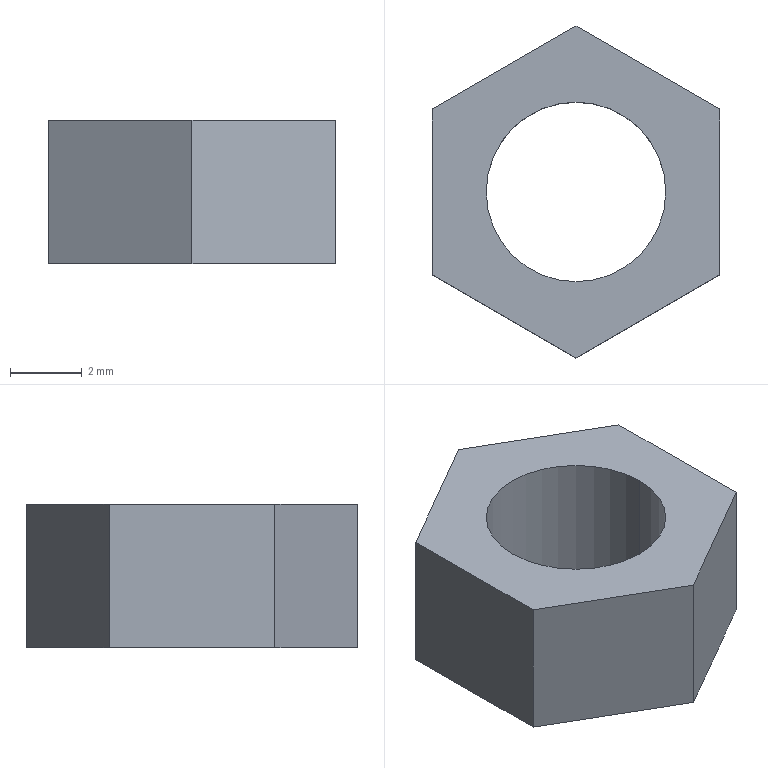Part | STEP file | M5 nut | 1 solid | 10 faces | box 8 x 9.238 x 4 mm | volume 143.163 mm3 | plane 8 | cylinder 2 | commonest cylinder face diameters 5 x2
STEP:
#1=CARTESIAN_POINT('',(0.,0.,0.));
#2=DIRECTION('',(0.,0.,1.));
#3=DIRECTION('',(1.,0.,0.));
#4=AXIS2_PLACEMENT_3D('',#1,#2,#3);
#5=CARTESIAN_POINT('',(2.5,0.,0.));
#6=VERTEX_POINT('',#5);
#7=CARTESIAN_POINT('',(2.5,0.,4.));
#8=VERTEX_POINT('',#7);
#9=CARTESIAN_POINT('',(2.5,0.,0.));
#10=DIRECTION('',(0.,0.,1.));
#11=VECTOR('',#10,1.);
#12=LINE('',#9,#11);
#13=CARTESIAN_POINT('',(0.,0.,0.));
#14=DIRECTION('',(0.,0.,1.));
#15=DIRECTION('',(1.,0.,0.));
#16=AXIS2_PLACEMENT_3D('',#13,#14,#15);
#17=CYLINDRICAL_SURFACE('',#16,2.5);
#18=CARTESIAN_POINT('',(6.283,0.));
#19=DIRECTION('',(0.,1.));
#20=VECTOR('',#19,1.);
#21=LINE('',#18,#20);
#22=(GEOMETRIC_REPRESENTATION_CONTEXT(2)PARAMETRIC_REPRESENTATION_CONTEXT()REPRESENTATION_CONTEXT('',''));
#23=DEFINITIONAL_REPRESENTATION('',(#21),#22);
#24=PCURVE('',#17,#23);
#25=CARTESIAN_POINT('',(0.,0.,0.));
#26=DIRECTION('',(0.,0.,1.));
#27=DIRECTION('',(1.,0.,0.));
#28=AXIS2_PLACEMENT_3D('',#25,#26,#27);
#29=CYLINDRICAL_SURFACE('',#28,2.5);
#30=CARTESIAN_POINT('',(0.,0.));
#31=DIRECTION('',(0.,1.));
#32=VECTOR('',#31,1.);
#33=LINE('',#30,#32);
#34=(GEOMETRIC_REPRESENTATION_CONTEXT(2)PARAMETRIC_REPRESENTATION_CONTEXT()REPRESENTATION_CONTEXT('',''));
#35=DEFINITIONAL_REPRESENTATION('',(#33),#34);
#36=PCURVE('',#29,#35);
#37=SURFACE_CURVE('',#12,(#24,#36),.PCURVE_S1.);
#38=EDGE_CURVE('',#6,#8,#37,.T.);
#39=ORIENTED_EDGE('',*,*,#38,.T.);
#40=CARTESIAN_POINT('',(-2.5,0.,4.));
#41=VERTEX_POINT('',#40);
#42=CARTESIAN_POINT('',(0.,0.,4.));
#43=DIRECTION('',(0.,0.,1.));
#44=DIRECTION('',(1.,0.,0.));
#45=AXIS2_PLACEMENT_3D('',#42,#43,#44);
#46=CIRCLE('',#45,2.5);
#47=CARTESIAN_POINT('',(0.,4.));
#48=DIRECTION('',(1.,0.));
#49=VECTOR('',#48,1.);
#50=LINE('',#47,#49);
#51=(GEOMETRIC_REPRESENTATION_CONTEXT(2)PARAMETRIC_REPRESENTATION_CONTEXT()REPRESENTATION_CONTEXT('',''));
#52=DEFINITIONAL_REPRESENTATION('',(#50),#51);
#53=PCURVE('',#17,#52);
#54=CARTESIAN_POINT('',(0.,0.,4.));
#55=DIRECTION('',(0.,0.,1.));
#56=DIRECTION('',(1.,0.,0.));
#57=AXIS2_PLACEMENT_3D('',#54,#55,#56);
#58=PLANE('',#57);
#59=CARTESIAN_POINT('',(0.,0.));
#60=DIRECTION('',(1.,0.));
#61=AXIS2_PLACEMENT_2D('',#59,#60);
#62=CIRCLE('',#61,2.5);
#63=(GEOMETRIC_REPRESENTATION_CONTEXT(2)PARAMETRIC_REPRESENTATION_CONTEXT()REPRESENTATION_CONTEXT('',''));
#64=DEFINITIONAL_REPRESENTATION('',(#62),#63);
#65=PCURVE('',#58,#64);
#66=SURFACE_CURVE('',#46,(#53,#65),.PCURVE_S1.);
#67=EDGE_CURVE('',#41,#8,#66,.T.);
#68=ORIENTED_EDGE('',*,*,#67,.F.);
#69=CARTESIAN_POINT('',(-2.5,0.,0.));
#70=VERTEX_POINT('',#69);
#71=CARTESIAN_POINT('',(-2.5,0.,0.));
#72=DIRECTION('',(0.,0.,1.));
#73=VECTOR('',#72,1.);
#74=LINE('',#71,#73);
#75=CARTESIAN_POINT('',(3.142,0.));
#76=DIRECTION('',(0.,1.));
#77=VECTOR('',#76,1.);
#78=LINE('',#75,#77);
#79=(GEOMETRIC_REPRESENTATION_CONTEXT(2)PARAMETRIC_REPRESENTATION_CONTEXT()REPRESENTATION_CONTEXT('',''));
#80=DEFINITIONAL_REPRESENTATION('',(#78),#79);
#81=PCURVE('',#17,#80);
#82=CARTESIAN_POINT('',(3.142,0.));
#83=DIRECTION('',(0.,1.));
#84=VECTOR('',#83,1.);
#85=LINE('',#82,#84);
#86=(GEOMETRIC_REPRESENTATION_CONTEXT(2)PARAMETRIC_REPRESENTATION_CONTEXT()REPRESENTATION_CONTEXT('',''));
#87=DEFINITIONAL_REPRESENTATION('',(#85),#86);
#88=PCURVE('',#29,#87);
#89=SURFACE_CURVE('',#74,(#81,#88),.PCURVE_S1.);
#90=EDGE_CURVE('',#70,#41,#89,.T.);
#91=ORIENTED_EDGE('',*,*,#90,.F.);
#92=CARTESIAN_POINT('',(0.,0.,0.));
#93=DIRECTION('',(0.,0.,1.));
#94=DIRECTION('',(1.,0.,0.));
#95=AXIS2_PLACEMENT_3D('',#92,#93,#94);
#96=CIRCLE('',#95,2.5);
#97=CARTESIAN_POINT('',(0.,0.));
#98=DIRECTION('',(1.,0.));
#99=VECTOR('',#98,1.);
#100=LINE('',#97,#99);
#101=(GEOMETRIC_REPRESENTATION_CONTEXT(2)PARAMETRIC_REPRESENTATION_CONTEXT()REPRESENTATION_CONTEXT('',''));
#102=DEFINITIONAL_REPRESENTATION('',(#100),#101);
#103=PCURVE('',#17,#102);
#104=CARTESIAN_POINT('',(0.,0.,0.));
#105=DIRECTION('',(0.,0.,1.));
#106=DIRECTION('',(1.,0.,0.));
#107=AXIS2_PLACEMENT_3D('',#104,#105,#106);
#108=PLANE('',#107);
#109=CARTESIAN_POINT('',(0.,0.));
#110=DIRECTION('',(1.,0.));
#111=AXIS2_PLACEMENT_2D('',#109,#110);
#112=CIRCLE('',#111,2.5);
#113=(GEOMETRIC_REPRESENTATION_CONTEXT(2)PARAMETRIC_REPRESENTATION_CONTEXT()REPRESENTATION_CONTEXT('',''));
#114=DEFINITIONAL_REPRESENTATION('',(#112),#113);
#115=PCURVE('',#108,#114);
#116=SURFACE_CURVE('',#96,(#103,#115),.PCURVE_S1.);
#117=EDGE_CURVE('',#70,#6,#116,.T.);
#118=ORIENTED_EDGE('',*,*,#117,.T.);
#119=EDGE_LOOP('',(#39,#68,#91,#118));
#120=FACE_BOUND('',#119,.F.);
#121=ADVANCED_FACE('',(#120),#17,.F.);
#122=CARTESIAN_POINT('',(-4.,2.309,0.));
#123=VERTEX_POINT('',#122);
#124=CARTESIAN_POINT('',(-4.,-2.309,0.));
#125=VERTEX_POINT('',#124);
#126=CARTESIAN_POINT('',(-4.,2.309,0.));
#127=DIRECTION('',(0.,-1.,0.));
#128=VECTOR('',#127,1.);
#129=LINE('',#126,#128);
#130=CARTESIAN_POINT('',(-4.,2.309,4.));
#131=DIRECTION('',(1.,0.,0.));
#132=DIRECTION('',(0.,0.,-1.));
#133=AXIS2_PLACEMENT_3D('',#130,#131,#132);
#134=PLANE('',#133);
#135=CARTESIAN_POINT('',(4.,0.));
#136=DIRECTION('',(0.,-1.));
#137=VECTOR('',#136,1.);
#138=LINE('',#135,#137);
#139=(GEOMETRIC_REPRESENTATION_CONTEXT(2)PARAMETRIC_REPRESENTATION_CONTEXT()REPRESENTATION_CONTEXT('',''));
#140=DEFINITIONAL_REPRESENTATION('',(#138),#139);
#141=PCURVE('',#134,#140);
#142=CARTESIAN_POINT('',(-4.,2.309));
#143=DIRECTION('',(0.,-1.));
#144=VECTOR('',#143,1.);
#145=LINE('',#142,#144);
#146=(GEOMETRIC_REPRESENTATION_CONTEXT(2)PARAMETRIC_REPRESENTATION_CONTEXT()REPRESENTATION_CONTEXT('',''));
#147=DEFINITIONAL_REPRESENTATION('',(#145),#146);
#148=PCURVE('',#108,#147);
#149=SURFACE_CURVE('',#129,(#141,#148),.PCURVE_S1.);
#150=EDGE_CURVE('',#123,#125,#149,.T.);
#151=ORIENTED_EDGE('',*,*,#150,.T.);
#152=CARTESIAN_POINT('',(-4.,-2.309,4.));
#153=VERTEX_POINT('',#152);
#154=CARTESIAN_POINT('',(-4.,-2.309,4.));
#155=DIRECTION('',(0.,0.,-1.));
#156=VECTOR('',#155,1.);
#157=LINE('',#154,#156);
#158=CARTESIAN_POINT('',(0.,-4.619));
#159=DIRECTION('',(1.,0.));
#160=VECTOR('',#159,1.);
#161=LINE('',#158,#160);
#162=(GEOMETRIC_REPRESENTATION_CONTEXT(2)PARAMETRIC_REPRESENTATION_CONTEXT()REPRESENTATION_CONTEXT('',''));
#163=DEFINITIONAL_REPRESENTATION('',(#161),#162);
#164=PCURVE('',#134,#163);
#165=CARTESIAN_POINT('',(-4.,-2.309,4.));
#166=DIRECTION('',(0.5,0.866,0.));
#167=DIRECTION('',(-0.866,0.5,0.));
#168=AXIS2_PLACEMENT_3D('',#165,#166,#167);
#169=PLANE('',#168);
#170=CARTESIAN_POINT('',(0.,0.));
#171=DIRECTION('',(0.,-1.));
#172=VECTOR('',#171,1.);
#173=LINE('',#170,#172);
#174=(GEOMETRIC_REPRESENTATION_CONTEXT(2)PARAMETRIC_REPRESENTATION_CONTEXT()REPRESENTATION_CONTEXT('',''));
#175=DEFINITIONAL_REPRESENTATION('',(#173),#174);
#176=PCURVE('',#169,#175);
#177=SURFACE_CURVE('',#157,(#164,#176),.PCURVE_S1.);
#178=EDGE_CURVE('',#153,#125,#177,.T.);
#179=ORIENTED_EDGE('',*,*,#178,.F.);
#180=CARTESIAN_POINT('',(-4.,2.309,4.));
#181=VERTEX_POINT('',#180);
#182=CARTESIAN_POINT('',(-4.,2.309,4.));
#183=DIRECTION('',(0.,-1.,0.));
#184=VECTOR('',#183,1.);
#185=LINE('',#182,#184);
#186=CARTESIAN_POINT('',(0.,0.));
#187=DIRECTION('',(0.,-1.));
#188=VECTOR('',#187,1.);
#189=LINE('',#186,#188);
#190=(GEOMETRIC_REPRESENTATION_CONTEXT(2)PARAMETRIC_REPRESENTATION_CONTEXT()REPRESENTATION_CONTEXT('',''));
#191=DEFINITIONAL_REPRESENTATION('',(#189),#190);
#192=PCURVE('',#134,#191);
#193=CARTESIAN_POINT('',(-4.,2.309));
#194=DIRECTION('',(0.,-1.));
#195=VECTOR('',#194,1.);
#196=LINE('',#193,#195);
#197=(GEOMETRIC_REPRESENTATION_CONTEXT(2)PARAMETRIC_REPRESENTATION_CONTEXT()REPRESENTATION_CONTEXT('',''));
#198=DEFINITIONAL_REPRESENTATION('',(#196),#197);
#199=PCURVE('',#58,#198);
#200=SURFACE_CURVE('',#185,(#192,#199),.PCURVE_S1.);
#201=EDGE_CURVE('',#181,#153,#200,.T.);
#202=ORIENTED_EDGE('',*,*,#201,.F.);
#203=CARTESIAN_POINT('',(-4.,2.309,4.));
#204=DIRECTION('',(0.,0.,-1.));
#205=VECTOR('',#204,1.);
#206=LINE('',#203,#205);
#207=CARTESIAN_POINT('',(0.,0.));
#208=DIRECTION('',(1.,0.));
#209=VECTOR('',#208,1.);
#210=LINE('',#207,#209);
#211=(GEOMETRIC_REPRESENTATION_CONTEXT(2)PARAMETRIC_REPRESENTATION_CONTEXT()REPRESENTATION_CONTEXT('',''));
#212=DEFINITIONAL_REPRESENTATION('',(#210),#211);
#213=PCURVE('',#134,#212);
#214=CARTESIAN_POINT('',(0.,4.619,4.));
#215=DIRECTION('',(0.5,-0.866,0.));
#216=DIRECTION('',(0.866,0.5,0.));
#217=AXIS2_PLACEMENT_3D('',#214,#215,#216);
#218=PLANE('',#217);
#219=CARTESIAN_POINT('',(-4.619,0.));
#220=DIRECTION('',(0.,-1.));
#221=VECTOR('',#220,1.);
#222=LINE('',#219,#221);
#223=(GEOMETRIC_REPRESENTATION_CONTEXT(2)PARAMETRIC_REPRESENTATION_CONTEXT()REPRESENTATION_CONTEXT('',''));
#224=DEFINITIONAL_REPRESENTATION('',(#222),#223);
#225=PCURVE('',#218,#224);
#226=SURFACE_CURVE('',#206,(#213,#225),.PCURVE_S1.);
#227=EDGE_CURVE('',#181,#123,#226,.T.);
#228=ORIENTED_EDGE('',*,*,#227,.T.);
#229=EDGE_LOOP('',(#151,#179,#202,#228));
#230=FACE_BOUND('',#229,.T.);
#231=ADVANCED_FACE('',(#230),#134,.F.);
#232=CARTESIAN_POINT('',(0.,-4.619,0.));
#233=VERTEX_POINT('',#232);
#234=CARTESIAN_POINT('',(-4.,-2.309,0.));
#235=DIRECTION('',(0.866,-0.5,0.));
#236=VECTOR('',#235,1.);
#237=LINE('',#234,#236);
#238=CARTESIAN_POINT('',(0.,-4.));
#239=DIRECTION('',(-1.,0.));
#240=VECTOR('',#239,1.);
#241=LINE('',#238,#240);
#242=(GEOMETRIC_REPRESENTATION_CONTEXT(2)PARAMETRIC_REPRESENTATION_CONTEXT()REPRESENTATION_CONTEXT('',''));
#243=DEFINITIONAL_REPRESENTATION('',(#241),#242);
#244=PCURVE('',#169,#243);
#245=CARTESIAN_POINT('',(-4.,-2.309));
#246=DIRECTION('',(0.866,-0.5));
#247=VECTOR('',#246,1.);
#248=LINE('',#245,#247);
#249=(GEOMETRIC_REPRESENTATION_CONTEXT(2)PARAMETRIC_REPRESENTATION_CONTEXT()REPRESENTATION_CONTEXT('',''));
#250=DEFINITIONAL_REPRESENTATION('',(#248),#249);
#251=PCURVE('',#108,#250);
#252=SURFACE_CURVE('',#237,(#244,#251),.PCURVE_S1.);
#253=EDGE_CURVE('',#125,#233,#252,.T.);
#254=ORIENTED_EDGE('',*,*,#253,.T.);
#255=CARTESIAN_POINT('',(0.,-4.619,4.));
#256=VERTEX_POINT('',#255);
#257=CARTESIAN_POINT('',(0.,-4.619,4.));
#258=DIRECTION('',(0.,0.,-1.));
#259=VECTOR('',#258,1.);
#260=LINE('',#257,#259);
#261=CARTESIAN_POINT('',(-4.619,0.));
#262=DIRECTION('',(0.,-1.));
#263=VECTOR('',#262,1.);
#264=LINE('',#261,#263);
#265=(GEOMETRIC_REPRESENTATION_CONTEXT(2)PARAMETRIC_REPRESENTATION_CONTEXT()REPRESENTATION_CONTEXT('',''));
#266=DEFINITIONAL_REPRESENTATION('',(#264),#265);
#267=PCURVE('',#169,#266);
#268=CARTESIAN_POINT('',(0.,-4.619,4.));
#269=DIRECTION('',(-0.5,0.866,0.));
#270=DIRECTION('',(-0.866,-0.5,0.));
#271=AXIS2_PLACEMENT_3D('',#268,#269,#270);
#272=PLANE('',#271);
#273=CARTESIAN_POINT('',(0.,0.));
#274=DIRECTION('',(0.,-1.));
#275=VECTOR('',#274,1.);
#276=LINE('',#273,#275);
#277=(GEOMETRIC_REPRESENTATION_CONTEXT(2)PARAMETRIC_REPRESENTATION_CONTEXT()REPRESENTATION_CONTEXT('',''));
#278=DEFINITIONAL_REPRESENTATION('',(#276),#277);
#279=PCURVE('',#272,#278);
#280=SURFACE_CURVE('',#260,(#267,#279),.PCURVE_S1.);
#281=EDGE_CURVE('',#256,#233,#280,.T.);
#282=ORIENTED_EDGE('',*,*,#281,.F.);
#283=CARTESIAN_POINT('',(-4.,-2.309,4.));
#284=DIRECTION('',(0.866,-0.5,0.));
#285=VECTOR('',#284,1.);
#286=LINE('',#283,#285);
#287=CARTESIAN_POINT('',(0.,0.));
#288=DIRECTION('',(-1.,0.));
#289=VECTOR('',#288,1.);
#290=LINE('',#287,#289);
#291=(GEOMETRIC_REPRESENTATION_CONTEXT(2)PARAMETRIC_REPRESENTATION_CONTEXT()REPRESENTATION_CONTEXT('',''));
#292=DEFINITIONAL_REPRESENTATION('',(#290),#291);
#293=PCURVE('',#169,#292);
#294=CARTESIAN_POINT('',(-4.,-2.309));
#295=DIRECTION('',(0.866,-0.5));
#296=VECTOR('',#295,1.);
#297=LINE('',#294,#296);
#298=(GEOMETRIC_REPRESENTATION_CONTEXT(2)PARAMETRIC_REPRESENTATION_CONTEXT()REPRESENTATION_CONTEXT('',''));
#299=DEFINITIONAL_REPRESENTATION('',(#297),#298);
#300=PCURVE('',#58,#299);
#301=SURFACE_CURVE('',#286,(#293,#300),.PCURVE_S1.);
#302=EDGE_CURVE('',#153,#256,#301,.T.);
#303=ORIENTED_EDGE('',*,*,#302,.F.);
#304=ORIENTED_EDGE('',*,*,#178,.T.);
#305=EDGE_LOOP('',(#254,#282,#303,#304));
#306=FACE_BOUND('',#305,.T.);
#307=ADVANCED_FACE('',(#306),#169,.F.);
#308=CARTESIAN_POINT('',(4.,-2.309,0.));
#309=VERTEX_POINT('',#308);
#310=CARTESIAN_POINT('',(0.,-4.619,0.));
#311=DIRECTION('',(0.866,0.5,0.));
#312=VECTOR('',#311,1.);
#313=LINE('',#310,#312);
#314=CARTESIAN_POINT('',(0.,-4.));
#315=DIRECTION('',(-1.,0.));
#316=VECTOR('',#315,1.);
#317=LINE('',#314,#316);
#318=(GEOMETRIC_REPRESENTATION_CONTEXT(2)PARAMETRIC_REPRESENTATION_CONTEXT()REPRESENTATION_CONTEXT('',''));
#319=DEFINITIONAL_REPRESENTATION('',(#317),#318);
#320=PCURVE('',#272,#319);
#321=CARTESIAN_POINT('',(0.,-4.619));
#322=DIRECTION('',(0.866,0.5));
#323=VECTOR('',#322,1.);
#324=LINE('',#321,#323);
#325=(GEOMETRIC_REPRESENTATION_CONTEXT(2)PARAMETRIC_REPRESENTATION_CONTEXT()REPRESENTATION_CONTEXT('',''));
#326=DEFINITIONAL_REPRESENTATION('',(#324),#325);
#327=PCURVE('',#108,#326);
#328=SURFACE_CURVE('',#313,(#320,#327),.PCURVE_S1.);
#329=EDGE_CURVE('',#233,#309,#328,.T.);
#330=ORIENTED_EDGE('',*,*,#329,.T.);
#331=CARTESIAN_POINT('',(4.,-2.309,4.));
#332=VERTEX_POINT('',#331);
#333=CARTESIAN_POINT('',(4.,-2.309,4.));
#334=DIRECTION('',(0.,0.,-1.));
#335=VECTOR('',#334,1.);
#336=LINE('',#333,#335);
#337=CARTESIAN_POINT('',(-4.619,0.));
#338=DIRECTION('',(0.,-1.));
#339=VECTOR('',#338,1.);
#340=LINE('',#337,#339);
#341=(GEOMETRIC_REPRESENTATION_CONTEXT(2)PARAMETRIC_REPRESENTATION_CONTEXT()REPRESENTATION_CONTEXT('',''));
#342=DEFINITIONAL_REPRESENTATION('',(#340),#341);
#343=PCURVE('',#272,#342);
#344=CARTESIAN_POINT('',(4.,-2.309,4.));
#345=DIRECTION('',(-1.,0.,0.));
#346=DIRECTION('',(0.,0.,1.));
#347=AXIS2_PLACEMENT_3D('',#344,#345,#346);
#348=PLANE('',#347);
#349=CARTESIAN_POINT('',(0.,0.));
#350=DIRECTION('',(-1.,0.));
#351=VECTOR('',#350,1.);
#352=LINE('',#349,#351);
#353=(GEOMETRIC_REPRESENTATION_CONTEXT(2)PARAMETRIC_REPRESENTATION_CONTEXT()REPRESENTATION_CONTEXT('',''));
#354=DEFINITIONAL_REPRESENTATION('',(#352),#353);
#355=PCURVE('',#348,#354);
#356=SURFACE_CURVE('',#336,(#343,#355),.PCURVE_S1.);
#357=EDGE_CURVE('',#332,#309,#356,.T.);
#358=ORIENTED_EDGE('',*,*,#357,.F.);
#359=CARTESIAN_POINT('',(0.,-4.619,4.));
#360=DIRECTION('',(0.866,0.5,0.));
#361=VECTOR('',#360,1.);
#362=LINE('',#359,#361);
#363=CARTESIAN_POINT('',(0.,0.));
#364=DIRECTION('',(-1.,0.));
#365=VECTOR('',#364,1.);
#366=LINE('',#363,#365);
#367=(GEOMETRIC_REPRESENTATION_CONTEXT(2)PARAMETRIC_REPRESENTATION_CONTEXT()REPRESENTATION_CONTEXT('',''));
#368=DEFINITIONAL_REPRESENTATION('',(#366),#367);
#369=PCURVE('',#272,#368);
#370=CARTESIAN_POINT('',(0.,-4.619));
#371=DIRECTION('',(0.866,0.5));
#372=VECTOR('',#371,1.);
#373=LINE('',#370,#372);
#374=(GEOMETRIC_REPRESENTATION_CONTEXT(2)PARAMETRIC_REPRESENTATION_CONTEXT()REPRESENTATION_CONTEXT('',''));
#375=DEFINITIONAL_REPRESENTATION('',(#373),#374);
#376=PCURVE('',#58,#375);
#377=SURFACE_CURVE('',#362,(#369,#376),.PCURVE_S1.);
#378=EDGE_CURVE('',#256,#332,#377,.T.);
#379=ORIENTED_EDGE('',*,*,#378,.F.);
#380=ORIENTED_EDGE('',*,*,#281,.T.);
#381=EDGE_LOOP('',(#330,#358,#379,#380));
#382=FACE_BOUND('',#381,.T.);
#383=ADVANCED_FACE('',(#382),#272,.F.);
#384=CARTESIAN_POINT('',(4.,2.309,0.));
#385=VERTEX_POINT('',#384);
#386=CARTESIAN_POINT('',(4.,-2.309,0.));
#387=DIRECTION('',(0.,1.,0.));
#388=VECTOR('',#387,1.);
#389=LINE('',#386,#388);
#390=CARTESIAN_POINT('',(-4.,0.));
#391=DIRECTION('',(0.,1.));
#392=VECTOR('',#391,1.);
#393=LINE('',#390,#392);
#394=(GEOMETRIC_REPRESENTATION_CONTEXT(2)PARAMETRIC_REPRESENTATION_CONTEXT()REPRESENTATION_CONTEXT('',''));
#395=DEFINITIONAL_REPRESENTATION('',(#393),#394);
#396=PCURVE('',#348,#395);
#397=CARTESIAN_POINT('',(4.,-2.309));
#398=DIRECTION('',(0.,1.));
#399=VECTOR('',#398,1.);
#400=LINE('',#397,#399);
#401=(GEOMETRIC_REPRESENTATION_CONTEXT(2)PARAMETRIC_REPRESENTATION_CONTEXT()REPRESENTATION_CONTEXT('',''));
#402=DEFINITIONAL_REPRESENTATION('',(#400),#401);
#403=PCURVE('',#108,#402);
#404=SURFACE_CURVE('',#389,(#396,#403),.PCURVE_S1.);
#405=EDGE_CURVE('',#309,#385,#404,.T.);
#406=ORIENTED_EDGE('',*,*,#405,.T.);
#407=CARTESIAN_POINT('',(4.,2.309,4.));
#408=VERTEX_POINT('',#407);
#409=CARTESIAN_POINT('',(4.,2.309,4.));
#410=DIRECTION('',(0.,0.,-1.));
#411=VECTOR('',#410,1.);
#412=LINE('',#409,#411);
#413=CARTESIAN_POINT('',(0.,4.619));
#414=DIRECTION('',(-1.,0.));
#415=VECTOR('',#414,1.);
#416=LINE('',#413,#415);
#417=(GEOMETRIC_REPRESENTATION_CONTEXT(2)PARAMETRIC_REPRESENTATION_CONTEXT()REPRESENTATION_CONTEXT('',''));
#418=DEFINITIONAL_REPRESENTATION('',(#416),#417);
#419=PCURVE('',#348,#418);
#420=CARTESIAN_POINT('',(4.,2.309,4.));
#421=DIRECTION('',(-0.5,-0.866,0.));
#422=DIRECTION('',(0.866,-0.5,0.));
#423=AXIS2_PLACEMENT_3D('',#420,#421,#422);
#424=PLANE('',#423);
#425=CARTESIAN_POINT('',(0.,0.));
#426=DIRECTION('',(0.,-1.));
#427=VECTOR('',#426,1.);
#428=LINE('',#425,#427);
#429=(GEOMETRIC_REPRESENTATION_CONTEXT(2)PARAMETRIC_REPRESENTATION_CONTEXT()REPRESENTATION_CONTEXT('',''));
#430=DEFINITIONAL_REPRESENTATION('',(#428),#429);
#431=PCURVE('',#424,#430);
#432=SURFACE_CURVE('',#412,(#419,#431),.PCURVE_S1.);
#433=EDGE_CURVE('',#408,#385,#432,.T.);
#434=ORIENTED_EDGE('',*,*,#433,.F.);
#435=CARTESIAN_POINT('',(4.,-2.309,4.));
#436=DIRECTION('',(0.,1.,0.));
#437=VECTOR('',#436,1.);
#438=LINE('',#435,#437);
#439=CARTESIAN_POINT('',(0.,0.));
#440=DIRECTION('',(0.,1.));
#441=VECTOR('',#440,1.);
#442=LINE('',#439,#441);
#443=(GEOMETRIC_REPRESENTATION_CONTEXT(2)PARAMETRIC_REPRESENTATION_CONTEXT()REPRESENTATION_CONTEXT('',''));
#444=DEFINITIONAL_REPRESENTATION('',(#442),#443);
#445=PCURVE('',#348,#444);
#446=CARTESIAN_POINT('',(4.,-2.309));
#447=DIRECTION('',(0.,1.));
#448=VECTOR('',#447,1.);
#449=LINE('',#446,#448);
#450=(GEOMETRIC_REPRESENTATION_CONTEXT(2)PARAMETRIC_REPRESENTATION_CONTEXT()REPRESENTATION_CONTEXT('',''));
#451=DEFINITIONAL_REPRESENTATION('',(#449),#450);
#452=PCURVE('',#58,#451);
#453=SURFACE_CURVE('',#438,(#445,#452),.PCURVE_S1.);
#454=EDGE_CURVE('',#332,#408,#453,.T.);
#455=ORIENTED_EDGE('',*,*,#454,.F.);
#456=ORIENTED_EDGE('',*,*,#357,.T.);
#457=EDGE_LOOP('',(#406,#434,#455,#456));
#458=FACE_BOUND('',#457,.T.);
#459=ADVANCED_FACE('',(#458),#348,.F.);
#460=CARTESIAN_POINT('',(0.,4.619,0.));
#461=VERTEX_POINT('',#460);
#462=CARTESIAN_POINT('',(4.,2.309,0.));
#463=DIRECTION('',(-0.866,0.5,0.));
#464=VECTOR('',#463,1.);
#465=LINE('',#462,#464);
#466=CARTESIAN_POINT('',(0.,-4.));
#467=DIRECTION('',(-1.,0.));
#468=VECTOR('',#467,1.);
#469=LINE('',#466,#468);
#470=(GEOMETRIC_REPRESENTATION_CONTEXT(2)PARAMETRIC_REPRESENTATION_CONTEXT()REPRESENTATION_CONTEXT('',''));
#471=DEFINITIONAL_REPRESENTATION('',(#469),#470);
#472=PCURVE('',#424,#471);
#473=CARTESIAN_POINT('',(4.,2.309));
#474=DIRECTION('',(-0.866,0.5));
#475=VECTOR('',#474,1.);
#476=LINE('',#473,#475);
#477=(GEOMETRIC_REPRESENTATION_CONTEXT(2)PARAMETRIC_REPRESENTATION_CONTEXT()REPRESENTATION_CONTEXT('',''));
#478=DEFINITIONAL_REPRESENTATION('',(#476),#477);
#479=PCURVE('',#108,#478);
#480=SURFACE_CURVE('',#465,(#472,#479),.PCURVE_S1.);
#481=EDGE_CURVE('',#385,#461,#480,.T.);
#482=ORIENTED_EDGE('',*,*,#481,.T.);
#483=CARTESIAN_POINT('',(0.,4.619,4.));
#484=VERTEX_POINT('',#483);
#485=CARTESIAN_POINT('',(0.,4.619,4.));
#486=DIRECTION('',(0.,0.,-1.));
#487=VECTOR('',#486,1.);
#488=LINE('',#485,#487);
#489=CARTESIAN_POINT('',(-4.619,0.));
#490=DIRECTION('',(0.,-1.));
#491=VECTOR('',#490,1.);
#492=LINE('',#489,#491);
#493=(GEOMETRIC_REPRESENTATION_CONTEXT(2)PARAMETRIC_REPRESENTATION_CONTEXT()REPRESENTATION_CONTEXT('',''));
#494=DEFINITIONAL_REPRESENTATION('',(#492),#493);
#495=PCURVE('',#424,#494);
#496=CARTESIAN_POINT('',(0.,0.));
#497=DIRECTION('',(0.,-1.));
#498=VECTOR('',#497,1.);
#499=LINE('',#496,#498);
#500=(GEOMETRIC_REPRESENTATION_CONTEXT(2)PARAMETRIC_REPRESENTATION_CONTEXT()REPRESENTATION_CONTEXT('',''));
#501=DEFINITIONAL_REPRESENTATION('',(#499),#500);
#502=PCURVE('',#218,#501);
#503=SURFACE_CURVE('',#488,(#495,#502),.PCURVE_S1.);
#504=EDGE_CURVE('',#484,#461,#503,.T.);
#505=ORIENTED_EDGE('',*,*,#504,.F.);
#506=CARTESIAN_POINT('',(4.,2.309,4.));
#507=DIRECTION('',(-0.866,0.5,0.));
#508=VECTOR('',#507,1.);
#509=LINE('',#506,#508);
#510=CARTESIAN_POINT('',(0.,0.));
#511=DIRECTION('',(-1.,0.));
#512=VECTOR('',#511,1.);
#513=LINE('',#510,#512);
#514=(GEOMETRIC_REPRESENTATION_CONTEXT(2)PARAMETRIC_REPRESENTATION_CONTEXT()REPRESENTATION_CONTEXT('',''));
#515=DEFINITIONAL_REPRESENTATION('',(#513),#514);
#516=PCURVE('',#424,#515);
#517=CARTESIAN_POINT('',(4.,2.309));
#518=DIRECTION('',(-0.866,0.5));
#519=VECTOR('',#518,1.);
#520=LINE('',#517,#519);
#521=(GEOMETRIC_REPRESENTATION_CONTEXT(2)PARAMETRIC_REPRESENTATION_CONTEXT()REPRESENTATION_CONTEXT('',''));
#522=DEFINITIONAL_REPRESENTATION('',(#520),#521);
#523=PCURVE('',#58,#522);
#524=SURFACE_CURVE('',#509,(#516,#523),.PCURVE_S1.);
#525=EDGE_CURVE('',#408,#484,#524,.T.);
#526=ORIENTED_EDGE('',*,*,#525,.F.);
#527=ORIENTED_EDGE('',*,*,#433,.T.);
#528=EDGE_LOOP('',(#482,#505,#526,#527));
#529=FACE_BOUND('',#528,.T.);
#530=ADVANCED_FACE('',(#529),#424,.F.);
#531=CARTESIAN_POINT('',(0.,4.619,0.));
#532=DIRECTION('',(-0.866,-0.5,0.));
#533=VECTOR('',#532,1.);
#534=LINE('',#531,#533);
#535=CARTESIAN_POINT('',(0.,-4.));
#536=DIRECTION('',(-1.,0.));
#537=VECTOR('',#536,1.);
#538=LINE('',#535,#537);
#539=(GEOMETRIC_REPRESENTATION_CONTEXT(2)PARAMETRIC_REPRESENTATION_CONTEXT()REPRESENTATION_CONTEXT('',''));
#540=DEFINITIONAL_REPRESENTATION('',(#538),#539);
#541=PCURVE('',#218,#540);
#542=CARTESIAN_POINT('',(0.,4.619));
#543=DIRECTION('',(-0.866,-0.5));
#544=VECTOR('',#543,1.);
#545=LINE('',#542,#544);
#546=(GEOMETRIC_REPRESENTATION_CONTEXT(2)PARAMETRIC_REPRESENTATION_CONTEXT()REPRESENTATION_CONTEXT('',''));
#547=DEFINITIONAL_REPRESENTATION('',(#545),#546);
#548=PCURVE('',#108,#547);
#549=SURFACE_CURVE('',#534,(#541,#548),.PCURVE_S1.);
#550=EDGE_CURVE('',#461,#123,#549,.T.);
#551=ORIENTED_EDGE('',*,*,#550,.T.);
#552=ORIENTED_EDGE('',*,*,#227,.F.);
#553=CARTESIAN_POINT('',(0.,4.619,4.));
#554=DIRECTION('',(-0.866,-0.5,0.));
#555=VECTOR('',#554,1.);
#556=LINE('',#553,#555);
#557=CARTESIAN_POINT('',(0.,0.));
#558=DIRECTION('',(-1.,0.));
#559=VECTOR('',#558,1.);
#560=LINE('',#557,#559);
#561=(GEOMETRIC_REPRESENTATION_CONTEXT(2)PARAMETRIC_REPRESENTATION_CONTEXT()REPRESENTATION_CONTEXT('',''));
#562=DEFINITIONAL_REPRESENTATION('',(#560),#561);
#563=PCURVE('',#218,#562);
#564=CARTESIAN_POINT('',(0.,4.619));
#565=DIRECTION('',(-0.866,-0.5));
#566=VECTOR('',#565,1.);
#567=LINE('',#564,#566);
#568=(GEOMETRIC_REPRESENTATION_CONTEXT(2)PARAMETRIC_REPRESENTATION_CONTEXT()REPRESENTATION_CONTEXT('',''));
#569=DEFINITIONAL_REPRESENTATION('',(#567),#568);
#570=PCURVE('',#58,#569);
#571=SURFACE_CURVE('',#556,(#563,#570),.PCURVE_S1.);
#572=EDGE_CURVE('',#484,#181,#571,.T.);
#573=ORIENTED_EDGE('',*,*,#572,.F.);
#574=ORIENTED_EDGE('',*,*,#504,.T.);
#575=EDGE_LOOP('',(#551,#552,#573,#574));
#576=FACE_BOUND('',#575,.T.);
#577=ADVANCED_FACE('',(#576),#218,.F.);
#578=CARTESIAN_POINT('',(0.,0.,4.));
#579=DIRECTION('',(0.,0.,1.));
#580=DIRECTION('',(1.,0.,0.));
#581=AXIS2_PLACEMENT_3D('',#578,#579,#580);
#582=CIRCLE('',#581,2.5);
#583=CARTESIAN_POINT('',(0.,0.));
#584=DIRECTION('',(1.,0.));
#585=AXIS2_PLACEMENT_2D('',#583,#584);
#586=CIRCLE('',#585,2.5);
#587=(GEOMETRIC_REPRESENTATION_CONTEXT(2)PARAMETRIC_REPRESENTATION_CONTEXT()REPRESENTATION_CONTEXT('',''));
#588=DEFINITIONAL_REPRESENTATION('',(#586),#587);
#589=PCURVE('',#58,#588);
#590=CARTESIAN_POINT('',(0.,4.));
#591=DIRECTION('',(1.,0.));
#592=VECTOR('',#591,1.);
#593=LINE('',#590,#592);
#594=(GEOMETRIC_REPRESENTATION_CONTEXT(2)PARAMETRIC_REPRESENTATION_CONTEXT()REPRESENTATION_CONTEXT('',''));
#595=DEFINITIONAL_REPRESENTATION('',(#593),#594);
#596=PCURVE('',#29,#595);
#597=SURFACE_CURVE('',#582,(#589,#596),.PCURVE_S1.);
#598=EDGE_CURVE('',#8,#41,#597,.T.);
#599=ORIENTED_EDGE('',*,*,#598,.F.);
#600=ORIENTED_EDGE('',*,*,#67,.F.);
#601=EDGE_LOOP('',(#599,#600));
#602=FACE_BOUND('',#601,.T.);
#603=ORIENTED_EDGE('',*,*,#201,.T.);
#604=ORIENTED_EDGE('',*,*,#302,.T.);
#605=ORIENTED_EDGE('',*,*,#378,.T.);
#606=ORIENTED_EDGE('',*,*,#454,.T.);
#607=ORIENTED_EDGE('',*,*,#525,.T.);
#608=ORIENTED_EDGE('',*,*,#572,.T.);
#609=EDGE_LOOP('',(#603,#604,#605,#606,#607,#608));
#610=FACE_BOUND('',#609,.T.);
#611=ADVANCED_FACE('',(#602,#610),#58,.T.);
#612=CARTESIAN_POINT('',(0.,0.,0.));
#613=DIRECTION('',(0.,0.,1.));
#614=DIRECTION('',(1.,0.,0.));
#615=AXIS2_PLACEMENT_3D('',#612,#613,#614);
#616=CIRCLE('',#615,2.5);
#617=CARTESIAN_POINT('',(0.,0.));
#618=DIRECTION('',(1.,0.));
#619=AXIS2_PLACEMENT_2D('',#617,#618);
#620=CIRCLE('',#619,2.5);
#621=(GEOMETRIC_REPRESENTATION_CONTEXT(2)PARAMETRIC_REPRESENTATION_CONTEXT()REPRESENTATION_CONTEXT('',''));
#622=DEFINITIONAL_REPRESENTATION('',(#620),#621);
#623=PCURVE('',#108,#622);
#624=CARTESIAN_POINT('',(0.,0.));
#625=DIRECTION('',(1.,0.));
#626=VECTOR('',#625,1.);
#627=LINE('',#624,#626);
#628=(GEOMETRIC_REPRESENTATION_CONTEXT(2)PARAMETRIC_REPRESENTATION_CONTEXT()REPRESENTATION_CONTEXT('',''));
#629=DEFINITIONAL_REPRESENTATION('',(#627),#628);
#630=PCURVE('',#29,#629);
#631=SURFACE_CURVE('',#616,(#623,#630),.PCURVE_S1.);
#632=EDGE_CURVE('',#6,#70,#631,.T.);
#633=ORIENTED_EDGE('',*,*,#632,.T.);
#634=ORIENTED_EDGE('',*,*,#117,.T.);
#635=EDGE_LOOP('',(#633,#634));
#636=FACE_BOUND('',#635,.T.);
#637=ORIENTED_EDGE('',*,*,#150,.F.);
#638=ORIENTED_EDGE('',*,*,#550,.F.);
#639=ORIENTED_EDGE('',*,*,#481,.F.);
#640=ORIENTED_EDGE('',*,*,#405,.F.);
#641=ORIENTED_EDGE('',*,*,#329,.F.);
#642=ORIENTED_EDGE('',*,*,#253,.F.);
#643=EDGE_LOOP('',(#637,#638,#639,#640,#641,#642));
#644=FACE_BOUND('',#643,.T.);
#645=ADVANCED_FACE('',(#636,#644),#108,.F.);
#646=ORIENTED_EDGE('',*,*,#598,.F.);
#647=ORIENTED_EDGE('',*,*,#38,.F.);
#648=ORIENTED_EDGE('',*,*,#632,.T.);
#649=ORIENTED_EDGE('',*,*,#90,.T.);
#650=EDGE_LOOP('',(#646,#647,#648,#649));
#651=FACE_BOUND('',#650,.F.);
#652=ADVANCED_FACE('',(#651),#29,.F.);
#653=CLOSED_SHELL('',(#121,#231,#307,#383,#459,#530,#577,#611,#645,#652));
#654=MANIFOLD_SOLID_BREP('',#653);
#655=(LENGTH_UNIT()NAMED_UNIT(*)SI_UNIT(.MILLI.,.METRE.));
#656=UNCERTAINTY_MEASURE_WITH_UNIT(LENGTH_MEASURE(0.0000001),#655,'','');
#657=(NAMED_UNIT(*)PLANE_ANGLE_UNIT()SI_UNIT($,.RADIAN.));
#658=(NAMED_UNIT(*)SI_UNIT($,.STERADIAN.)SOLID_ANGLE_UNIT());
#659=(GEOMETRIC_REPRESENTATION_CONTEXT(3)GLOBAL_UNCERTAINTY_ASSIGNED_CONTEXT((#656))GLOBAL_UNIT_ASSIGNED_CONTEXT((#655,#657,#658))REPRESENTATION_CONTEXT('',''));
#660=ADVANCED_BREP_SHAPE_REPRESENTATION('',(#4,#654),#659);